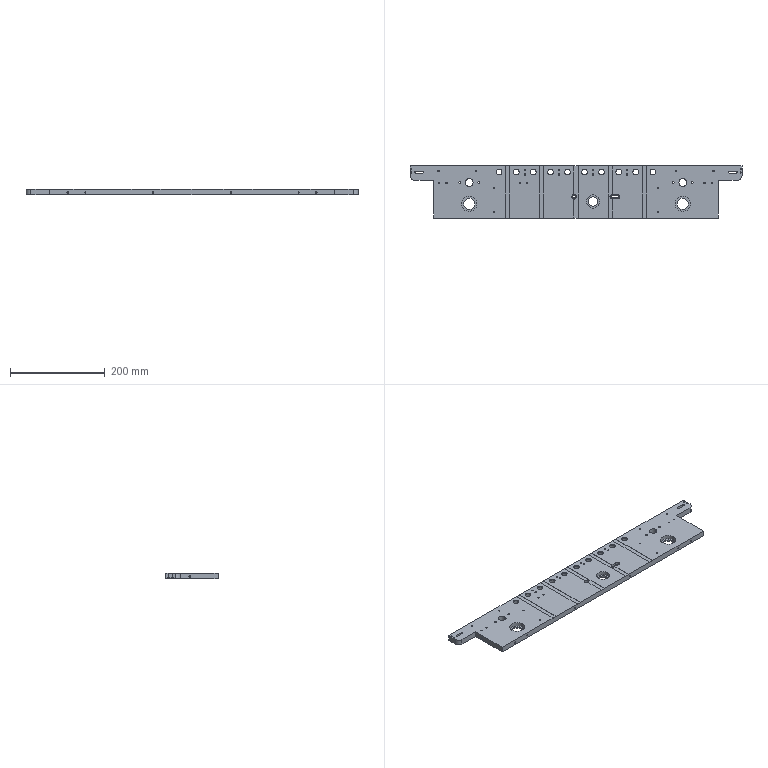Part | SolidWorks | features HoleWzd 15, ICE 11, Cut 1, Extrusion 1, Fillet 1 | 1 solid | 273 faces | box 700 x 110 x 12 mm | volume 766656 mm3 | cylinder 194 | plane 59 | cone 20 | commonest cylinder face diameters 2.5 x52 3.3 x44 16 x24 12 x20 2.4 x8 4.2 x8